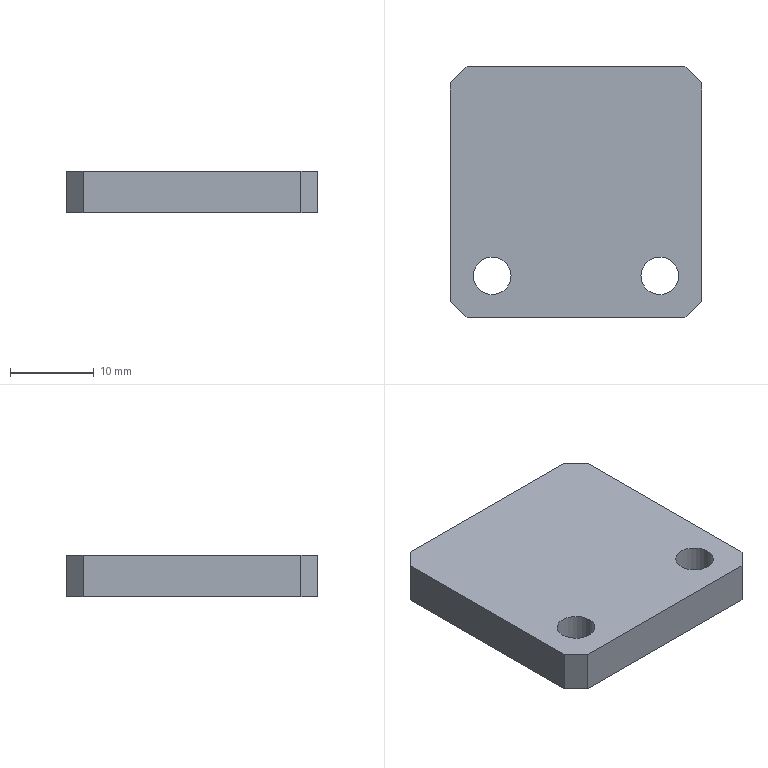Part | STEP file | 01-12 front baffle | 1 solid | 14 faces | box 30 x 30 x 5 mm | volume 4301 mm3 | plane 10 | cylinder 4 | commonest cylinder face diameters 4.5 x4
STEP:
#1=CARTESIAN_POINT('',(7.75,-10.,0.));
#2=VERTEX_POINT('',#1);
#3=CARTESIAN_POINT('',(12.25,-10.,0.));
#4=VERTEX_POINT('',#3);
#5=CARTESIAN_POINT('',(10.,-10.,0.));
#6=DIRECTION('',(0.,0.,1.));
#7=DIRECTION('',(1.,0.,0.));
#8=AXIS2_PLACEMENT_3D('',#5,#6,#7);
#9=CIRCLE('',#8,2.25);
#10=EDGE_CURVE('',#2,#4,#9,.T.);
#11=ORIENTED_EDGE('',*,*,#10,.F.);
#12=CARTESIAN_POINT('',(7.75,-10.,5.));
#13=VERTEX_POINT('',#12);
#14=CARTESIAN_POINT('',(7.75,-10.,0.));
#15=DIRECTION('',(0.,0.,1.));
#16=VECTOR('',#15,1000.);
#17=LINE('',#14,#16);
#18=EDGE_CURVE('',#2,#13,#17,.T.);
#19=ORIENTED_EDGE('',*,*,#18,.T.);
#20=CARTESIAN_POINT('',(12.25,-10.,5.));
#21=VERTEX_POINT('',#20);
#22=CARTESIAN_POINT('',(10.,-10.,5.));
#23=DIRECTION('',(0.,0.,1.));
#24=DIRECTION('',(1.,0.,0.));
#25=AXIS2_PLACEMENT_3D('',#22,#23,#24);
#26=CIRCLE('',#25,2.25);
#27=EDGE_CURVE('',#13,#21,#26,.T.);
#28=ORIENTED_EDGE('',*,*,#27,.T.);
#29=CARTESIAN_POINT('',(12.25,-10.,0.));
#30=DIRECTION('',(0.,0.,1.));
#31=VECTOR('',#30,1000.);
#32=LINE('',#29,#31);
#33=EDGE_CURVE('',#4,#21,#32,.T.);
#34=ORIENTED_EDGE('',*,*,#33,.F.);
#35=EDGE_LOOP('',(#11,#19,#28,#34));
#36=FACE_OUTER_BOUND('',#35,.T.);
#37=CARTESIAN_POINT('',(10.,-10.,0.));
#38=DIRECTION('',(0.,0.,1.));
#39=DIRECTION('',(1.,0.,0.));
#40=AXIS2_PLACEMENT_3D('',#37,#38,#39);
#41=CYLINDRICAL_SURFACE('',#40,2.25);
#42=ADVANCED_FACE('',(#36),#41,.F.);
#43=CARTESIAN_POINT('',(-12.25,-10.,0.));
#44=VERTEX_POINT('',#43);
#45=CARTESIAN_POINT('',(-7.75,-10.,0.));
#46=VERTEX_POINT('',#45);
#47=CARTESIAN_POINT('',(-10.,-10.,0.));
#48=DIRECTION('',(0.,0.,1.));
#49=DIRECTION('',(1.,0.,0.));
#50=AXIS2_PLACEMENT_3D('',#47,#48,#49);
#51=CIRCLE('',#50,2.25);
#52=EDGE_CURVE('',#44,#46,#51,.T.);
#53=ORIENTED_EDGE('',*,*,#52,.F.);
#54=CARTESIAN_POINT('',(-12.25,-10.,5.));
#55=VERTEX_POINT('',#54);
#56=CARTESIAN_POINT('',(-12.25,-10.,0.));
#57=DIRECTION('',(0.,0.,1.));
#58=VECTOR('',#57,1000.);
#59=LINE('',#56,#58);
#60=EDGE_CURVE('',#44,#55,#59,.T.);
#61=ORIENTED_EDGE('',*,*,#60,.T.);
#62=CARTESIAN_POINT('',(-7.75,-10.,5.));
#63=VERTEX_POINT('',#62);
#64=CARTESIAN_POINT('',(-10.,-10.,5.));
#65=DIRECTION('',(0.,0.,1.));
#66=DIRECTION('',(1.,0.,0.));
#67=AXIS2_PLACEMENT_3D('',#64,#65,#66);
#68=CIRCLE('',#67,2.25);
#69=EDGE_CURVE('',#55,#63,#68,.T.);
#70=ORIENTED_EDGE('',*,*,#69,.T.);
#71=CARTESIAN_POINT('',(-7.75,-10.,0.));
#72=DIRECTION('',(0.,0.,1.));
#73=VECTOR('',#72,1000.);
#74=LINE('',#71,#73);
#75=EDGE_CURVE('',#46,#63,#74,.T.);
#76=ORIENTED_EDGE('',*,*,#75,.F.);
#77=EDGE_LOOP('',(#53,#61,#70,#76));
#78=FACE_OUTER_BOUND('',#77,.T.);
#79=CARTESIAN_POINT('',(-10.,-10.,0.));
#80=DIRECTION('',(0.,0.,1.));
#81=DIRECTION('',(1.,0.,0.));
#82=AXIS2_PLACEMENT_3D('',#79,#80,#81);
#83=CYLINDRICAL_SURFACE('',#82,2.25);
#84=ADVANCED_FACE('',(#78),#83,.F.);
#85=CARTESIAN_POINT('',(15.,-13.,5.));
#86=VERTEX_POINT('',#85);
#87=CARTESIAN_POINT('',(15.,13.,5.));
#88=VERTEX_POINT('',#87);
#89=CARTESIAN_POINT('',(15.,15.,5.));
#90=DIRECTION('',(0.,1.,0.));
#91=VECTOR('',#90,1000.);
#92=LINE('',#89,#91);
#93=EDGE_CURVE('',#86,#88,#92,.T.);
#94=ORIENTED_EDGE('',*,*,#93,.F.);
#95=CARTESIAN_POINT('',(15.,-13.,0.));
#96=VERTEX_POINT('',#95);
#97=CARTESIAN_POINT('',(15.,-13.,5.));
#98=DIRECTION('',(0.,0.,-1.));
#99=VECTOR('',#98,1000.);
#100=LINE('',#97,#99);
#101=EDGE_CURVE('',#86,#96,#100,.T.);
#102=ORIENTED_EDGE('',*,*,#101,.T.);
#103=CARTESIAN_POINT('',(15.,13.,0.));
#104=VERTEX_POINT('',#103);
#105=CARTESIAN_POINT('',(15.,15.,0.));
#106=DIRECTION('',(0.,1.,0.));
#107=VECTOR('',#106,1000.);
#108=LINE('',#105,#107);
#109=EDGE_CURVE('',#96,#104,#108,.T.);
#110=ORIENTED_EDGE('',*,*,#109,.T.);
#111=CARTESIAN_POINT('',(15.,13.,5.));
#112=DIRECTION('',(0.,0.,1.));
#113=VECTOR('',#112,1000.);
#114=LINE('',#111,#113);
#115=EDGE_CURVE('',#104,#88,#114,.T.);
#116=ORIENTED_EDGE('',*,*,#115,.T.);
#117=EDGE_LOOP('',(#94,#102,#110,#116));
#118=FACE_OUTER_BOUND('',#117,.T.);
#119=CARTESIAN_POINT('',(15.,15.,5.));
#120=DIRECTION('',(-1.,0.,0.));
#121=DIRECTION('',(0.,-1.,0.));
#122=AXIS2_PLACEMENT_3D('',#119,#120,#121);
#123=PLANE('',#122);
#124=ADVANCED_FACE('',(#118),#123,.F.);
#125=CARTESIAN_POINT('',(13.,15.,5.));
#126=VERTEX_POINT('',#125);
#127=CARTESIAN_POINT('',(-13.,15.,5.));
#128=VERTEX_POINT('',#127);
#129=CARTESIAN_POINT('',(-15.,15.,5.));
#130=DIRECTION('',(-1.,0.,0.));
#131=VECTOR('',#130,1000.);
#132=LINE('',#129,#131);
#133=EDGE_CURVE('',#126,#128,#132,.T.);
#134=ORIENTED_EDGE('',*,*,#133,.F.);
#135=CARTESIAN_POINT('',(13.,15.,0.));
#136=VERTEX_POINT('',#135);
#137=CARTESIAN_POINT('',(13.,15.,5.));
#138=DIRECTION('',(0.,0.,-1.));
#139=VECTOR('',#138,1000.);
#140=LINE('',#137,#139);
#141=EDGE_CURVE('',#126,#136,#140,.T.);
#142=ORIENTED_EDGE('',*,*,#141,.T.);
#143=CARTESIAN_POINT('',(-13.,15.,0.));
#144=VERTEX_POINT('',#143);
#145=CARTESIAN_POINT('',(-15.,15.,0.));
#146=DIRECTION('',(-1.,0.,0.));
#147=VECTOR('',#146,1000.);
#148=LINE('',#145,#147);
#149=EDGE_CURVE('',#136,#144,#148,.T.);
#150=ORIENTED_EDGE('',*,*,#149,.T.);
#151=CARTESIAN_POINT('',(-13.,15.,5.));
#152=DIRECTION('',(0.,0.,1.));
#153=VECTOR('',#152,1000.);
#154=LINE('',#151,#153);
#155=EDGE_CURVE('',#144,#128,#154,.T.);
#156=ORIENTED_EDGE('',*,*,#155,.T.);
#157=EDGE_LOOP('',(#134,#142,#150,#156));
#158=FACE_OUTER_BOUND('',#157,.T.);
#159=CARTESIAN_POINT('',(-15.,15.,5.));
#160=DIRECTION('',(0.,-1.,0.));
#161=DIRECTION('',(0.,0.,-1.));
#162=AXIS2_PLACEMENT_3D('',#159,#160,#161);
#163=PLANE('',#162);
#164=ADVANCED_FACE('',(#158),#163,.F.);
#165=CARTESIAN_POINT('',(-15.,13.,0.));
#166=VERTEX_POINT('',#165);
#167=CARTESIAN_POINT('',(-15.,-13.,0.));
#168=VERTEX_POINT('',#167);
#169=CARTESIAN_POINT('',(-15.,15.,0.));
#170=DIRECTION('',(0.,-1.,0.));
#171=VECTOR('',#170,1000.);
#172=LINE('',#169,#171);
#173=EDGE_CURVE('',#166,#168,#172,.T.);
#174=ORIENTED_EDGE('',*,*,#173,.T.);
#175=CARTESIAN_POINT('',(-15.,-13.,5.));
#176=VERTEX_POINT('',#175);
#177=CARTESIAN_POINT('',(-15.,-13.,5.));
#178=DIRECTION('',(0.,0.,1.));
#179=VECTOR('',#178,1000.);
#180=LINE('',#177,#179);
#181=EDGE_CURVE('',#168,#176,#180,.T.);
#182=ORIENTED_EDGE('',*,*,#181,.T.);
#183=CARTESIAN_POINT('',(-15.,13.,5.));
#184=VERTEX_POINT('',#183);
#185=CARTESIAN_POINT('',(-15.,15.,5.));
#186=DIRECTION('',(0.,-1.,0.));
#187=VECTOR('',#186,1000.);
#188=LINE('',#185,#187);
#189=EDGE_CURVE('',#184,#176,#188,.T.);
#190=ORIENTED_EDGE('',*,*,#189,.F.);
#191=CARTESIAN_POINT('',(-15.,13.,5.));
#192=DIRECTION('',(0.,0.,-1.));
#193=VECTOR('',#192,1000.);
#194=LINE('',#191,#193);
#195=EDGE_CURVE('',#184,#166,#194,.T.);
#196=ORIENTED_EDGE('',*,*,#195,.T.);
#197=EDGE_LOOP('',(#174,#182,#190,#196));
#198=FACE_OUTER_BOUND('',#197,.T.);
#199=CARTESIAN_POINT('',(-15.,15.,5.));
#200=DIRECTION('',(1.,0.,0.));
#201=DIRECTION('',(0.,1.,0.));
#202=AXIS2_PLACEMENT_3D('',#199,#200,#201);
#203=PLANE('',#202);
#204=ADVANCED_FACE('',(#198),#203,.F.);
#205=CARTESIAN_POINT('',(-13.,-15.,0.));
#206=VERTEX_POINT('',#205);
#207=CARTESIAN_POINT('',(13.,-15.,0.));
#208=VERTEX_POINT('',#207);
#209=CARTESIAN_POINT('',(-15.,-15.,0.));
#210=DIRECTION('',(1.,0.,0.));
#211=VECTOR('',#210,1000.);
#212=LINE('',#209,#211);
#213=EDGE_CURVE('',#206,#208,#212,.T.);
#214=ORIENTED_EDGE('',*,*,#213,.T.);
#215=CARTESIAN_POINT('',(13.,-15.,5.));
#216=VERTEX_POINT('',#215);
#217=CARTESIAN_POINT('',(13.,-15.,5.));
#218=DIRECTION('',(0.,0.,1.));
#219=VECTOR('',#218,1000.);
#220=LINE('',#217,#219);
#221=EDGE_CURVE('',#208,#216,#220,.T.);
#222=ORIENTED_EDGE('',*,*,#221,.T.);
#223=CARTESIAN_POINT('',(-13.,-15.,5.));
#224=VERTEX_POINT('',#223);
#225=CARTESIAN_POINT('',(-15.,-15.,5.));
#226=DIRECTION('',(1.,0.,0.));
#227=VECTOR('',#226,1000.);
#228=LINE('',#225,#227);
#229=EDGE_CURVE('',#224,#216,#228,.T.);
#230=ORIENTED_EDGE('',*,*,#229,.F.);
#231=CARTESIAN_POINT('',(-13.,-15.,5.));
#232=DIRECTION('',(0.,0.,-1.));
#233=VECTOR('',#232,1000.);
#234=LINE('',#231,#233);
#235=EDGE_CURVE('',#224,#206,#234,.T.);
#236=ORIENTED_EDGE('',*,*,#235,.T.);
#237=EDGE_LOOP('',(#214,#222,#230,#236));
#238=FACE_OUTER_BOUND('',#237,.T.);
#239=CARTESIAN_POINT('',(-15.,-15.,5.));
#240=DIRECTION('',(0.,1.,0.));
#241=DIRECTION('',(0.,0.,1.));
#242=AXIS2_PLACEMENT_3D('',#239,#240,#241);
#243=PLANE('',#242);
#244=ADVANCED_FACE('',(#238),#243,.F.);
#245=CARTESIAN_POINT('',(10.,-10.,5.));
#246=DIRECTION('',(0.,0.,1.));
#247=DIRECTION('',(1.,0.,0.));
#248=AXIS2_PLACEMENT_3D('',#245,#246,#247);
#249=CIRCLE('',#248,2.25);
#250=EDGE_CURVE('',#21,#13,#249,.T.);
#251=ORIENTED_EDGE('',*,*,#250,.F.);
#252=ORIENTED_EDGE('',*,*,#27,.F.);
#253=EDGE_LOOP('',(#251,#252));
#254=FACE_BOUND('',#253,.T.);
#255=CARTESIAN_POINT('',(-10.,-10.,5.));
#256=DIRECTION('',(0.,0.,1.));
#257=DIRECTION('',(1.,0.,0.));
#258=AXIS2_PLACEMENT_3D('',#255,#256,#257);
#259=CIRCLE('',#258,2.25);
#260=EDGE_CURVE('',#63,#55,#259,.T.);
#261=ORIENTED_EDGE('',*,*,#260,.F.);
#262=ORIENTED_EDGE('',*,*,#69,.F.);
#263=EDGE_LOOP('',(#261,#262));
#264=FACE_BOUND('',#263,.T.);
#265=ORIENTED_EDGE('',*,*,#229,.T.);
#266=CARTESIAN_POINT('',(14.,-14.,5.));
#267=DIRECTION('',(0.7071,0.7071,0.));
#268=VECTOR('',#267,1000.);
#269=LINE('',#266,#268);
#270=EDGE_CURVE('',#216,#86,#269,.T.);
#271=ORIENTED_EDGE('',*,*,#270,.T.);
#272=ORIENTED_EDGE('',*,*,#93,.T.);
#273=CARTESIAN_POINT('',(29.,-1.,5.));
#274=DIRECTION('',(-0.7071,0.7071,0.));
#275=VECTOR('',#274,1000.);
#276=LINE('',#273,#275);
#277=EDGE_CURVE('',#88,#126,#276,.T.);
#278=ORIENTED_EDGE('',*,*,#277,.T.);
#279=ORIENTED_EDGE('',*,*,#133,.T.);
#280=CARTESIAN_POINT('',(-14.,14.,5.));
#281=DIRECTION('',(-0.7071,-0.7071,0.));
#282=VECTOR('',#281,1000.);
#283=LINE('',#280,#282);
#284=EDGE_CURVE('',#128,#184,#283,.T.);
#285=ORIENTED_EDGE('',*,*,#284,.T.);
#286=ORIENTED_EDGE('',*,*,#189,.T.);
#287=CARTESIAN_POINT('',(1.,-29.,5.));
#288=DIRECTION('',(0.7071,-0.7071,0.));
#289=VECTOR('',#288,1000.);
#290=LINE('',#287,#289);
#291=EDGE_CURVE('',#176,#224,#290,.T.);
#292=ORIENTED_EDGE('',*,*,#291,.T.);
#293=EDGE_LOOP('',(#265,#271,#272,#278,#279,#285,#286,#292));
#294=FACE_OUTER_BOUND('',#293,.T.);
#295=CARTESIAN_POINT('',(15.,-15.,5.));
#296=DIRECTION('',(0.,0.,1.));
#297=DIRECTION('',(1.,0.,0.));
#298=AXIS2_PLACEMENT_3D('',#295,#296,#297);
#299=PLANE('',#298);
#300=ADVANCED_FACE('',(#254,#264,#294),#299,.T.);
#301=CARTESIAN_POINT('',(10.,-10.,0.));
#302=DIRECTION('',(0.,0.,1.));
#303=DIRECTION('',(1.,0.,0.));
#304=AXIS2_PLACEMENT_3D('',#301,#302,#303);
#305=CIRCLE('',#304,2.25);
#306=EDGE_CURVE('',#4,#2,#305,.T.);
#307=ORIENTED_EDGE('',*,*,#306,.T.);
#308=ORIENTED_EDGE('',*,*,#10,.T.);
#309=EDGE_LOOP('',(#307,#308));
#310=FACE_BOUND('',#309,.T.);
#311=CARTESIAN_POINT('',(-10.,-10.,0.));
#312=DIRECTION('',(0.,0.,1.));
#313=DIRECTION('',(1.,0.,0.));
#314=AXIS2_PLACEMENT_3D('',#311,#312,#313);
#315=CIRCLE('',#314,2.25);
#316=EDGE_CURVE('',#46,#44,#315,.T.);
#317=ORIENTED_EDGE('',*,*,#316,.T.);
#318=ORIENTED_EDGE('',*,*,#52,.T.);
#319=EDGE_LOOP('',(#317,#318));
#320=FACE_BOUND('',#319,.T.);
#321=ORIENTED_EDGE('',*,*,#109,.F.);
#322=CARTESIAN_POINT('',(15.,-13.,0.));
#323=DIRECTION('',(-0.7071,-0.7071,0.));
#324=VECTOR('',#323,1000.);
#325=LINE('',#322,#324);
#326=EDGE_CURVE('',#96,#208,#325,.T.);
#327=ORIENTED_EDGE('',*,*,#326,.T.);
#328=ORIENTED_EDGE('',*,*,#213,.F.);
#329=CARTESIAN_POINT('',(-13.,-15.,0.));
#330=DIRECTION('',(-0.7071,0.7071,0.));
#331=VECTOR('',#330,1000.);
#332=LINE('',#329,#331);
#333=EDGE_CURVE('',#206,#168,#332,.T.);
#334=ORIENTED_EDGE('',*,*,#333,.T.);
#335=ORIENTED_EDGE('',*,*,#173,.F.);
#336=CARTESIAN_POINT('',(-15.,13.,0.));
#337=DIRECTION('',(0.7071,0.7071,0.));
#338=VECTOR('',#337,1000.);
#339=LINE('',#336,#338);
#340=EDGE_CURVE('',#166,#144,#339,.T.);
#341=ORIENTED_EDGE('',*,*,#340,.T.);
#342=ORIENTED_EDGE('',*,*,#149,.F.);
#343=CARTESIAN_POINT('',(13.,15.,0.));
#344=DIRECTION('',(0.7071,-0.7071,0.));
#345=VECTOR('',#344,1000.);
#346=LINE('',#343,#345);
#347=EDGE_CURVE('',#136,#104,#346,.T.);
#348=ORIENTED_EDGE('',*,*,#347,.T.);
#349=EDGE_LOOP('',(#321,#327,#328,#334,#335,#341,#342,#348));
#350=FACE_OUTER_BOUND('',#349,.T.);
#351=CARTESIAN_POINT('',(15.,-15.,0.));
#352=DIRECTION('',(0.,0.,1.));
#353=DIRECTION('',(1.,0.,0.));
#354=AXIS2_PLACEMENT_3D('',#351,#352,#353);
#355=PLANE('',#354);
#356=ADVANCED_FACE('',(#310,#320,#350),#355,.F.);
#357=ORIENTED_EDGE('',*,*,#270,.F.);
#358=ORIENTED_EDGE('',*,*,#221,.F.);
#359=ORIENTED_EDGE('',*,*,#326,.F.);
#360=ORIENTED_EDGE('',*,*,#101,.F.);
#361=EDGE_LOOP('',(#357,#358,#359,#360));
#362=FACE_OUTER_BOUND('',#361,.T.);
#363=CARTESIAN_POINT('',(15.,-13.,5.));
#364=DIRECTION('',(-0.7071,0.7071,0.));
#365=DIRECTION('',(-0.7071,-0.7071,0.));
#366=AXIS2_PLACEMENT_3D('',#363,#364,#365);
#367=PLANE('',#366);
#368=ADVANCED_FACE('',(#362),#367,.F.);
#369=ORIENTED_EDGE('',*,*,#291,.F.);
#370=ORIENTED_EDGE('',*,*,#181,.F.);
#371=ORIENTED_EDGE('',*,*,#333,.F.);
#372=ORIENTED_EDGE('',*,*,#235,.F.);
#373=EDGE_LOOP('',(#369,#370,#371,#372));
#374=FACE_OUTER_BOUND('',#373,.T.);
#375=CARTESIAN_POINT('',(-13.,-15.,5.));
#376=DIRECTION('',(0.7071,0.7071,0.));
#377=DIRECTION('',(-0.7071,0.7071,0.));
#378=AXIS2_PLACEMENT_3D('',#375,#376,#377);
#379=PLANE('',#378);
#380=ADVANCED_FACE('',(#374),#379,.F.);
#381=ORIENTED_EDGE('',*,*,#277,.F.);
#382=ORIENTED_EDGE('',*,*,#115,.F.);
#383=ORIENTED_EDGE('',*,*,#347,.F.);
#384=ORIENTED_EDGE('',*,*,#141,.F.);
#385=EDGE_LOOP('',(#381,#382,#383,#384));
#386=FACE_OUTER_BOUND('',#385,.T.);
#387=CARTESIAN_POINT('',(13.,15.,5.));
#388=DIRECTION('',(-0.7071,-0.7071,0.));
#389=DIRECTION('',(0.7071,-0.7071,0.));
#390=AXIS2_PLACEMENT_3D('',#387,#388,#389);
#391=PLANE('',#390);
#392=ADVANCED_FACE('',(#386),#391,.F.);
#393=ORIENTED_EDGE('',*,*,#284,.F.);
#394=ORIENTED_EDGE('',*,*,#155,.F.);
#395=ORIENTED_EDGE('',*,*,#340,.F.);
#396=ORIENTED_EDGE('',*,*,#195,.F.);
#397=EDGE_LOOP('',(#393,#394,#395,#396));
#398=FACE_OUTER_BOUND('',#397,.T.);
#399=CARTESIAN_POINT('',(-15.,13.,5.));
#400=DIRECTION('',(0.7071,-0.7071,0.));
#401=DIRECTION('',(0.7071,0.7071,0.));
#402=AXIS2_PLACEMENT_3D('',#399,#400,#401);
#403=PLANE('',#402);
#404=ADVANCED_FACE('',(#398),#403,.F.);
#405=ORIENTED_EDGE('',*,*,#60,.F.);
#406=ORIENTED_EDGE('',*,*,#316,.F.);
#407=ORIENTED_EDGE('',*,*,#75,.T.);
#408=ORIENTED_EDGE('',*,*,#260,.T.);
#409=EDGE_LOOP('',(#405,#406,#407,#408));
#410=FACE_OUTER_BOUND('',#409,.T.);
#411=CARTESIAN_POINT('',(-10.,-10.,0.));
#412=DIRECTION('',(0.,0.,1.));
#413=DIRECTION('',(1.,0.,0.));
#414=AXIS2_PLACEMENT_3D('',#411,#412,#413);
#415=CYLINDRICAL_SURFACE('',#414,2.25);
#416=ADVANCED_FACE('',(#410),#415,.F.);
#417=ORIENTED_EDGE('',*,*,#18,.F.);
#418=ORIENTED_EDGE('',*,*,#306,.F.);
#419=ORIENTED_EDGE('',*,*,#33,.T.);
#420=ORIENTED_EDGE('',*,*,#250,.T.);
#421=EDGE_LOOP('',(#417,#418,#419,#420));
#422=FACE_OUTER_BOUND('',#421,.T.);
#423=CARTESIAN_POINT('',(10.,-10.,0.));
#424=DIRECTION('',(0.,0.,1.));
#425=DIRECTION('',(1.,0.,0.));
#426=AXIS2_PLACEMENT_3D('',#423,#424,#425);
#427=CYLINDRICAL_SURFACE('',#426,2.25);
#428=ADVANCED_FACE('',(#422),#427,.F.);
#429=CLOSED_SHELL('',(#42,#84,#124,#164,#204,#244,#300,#356,#368,#380,#392,#404,#416,#428));
#430=MANIFOLD_SOLID_BREP('',#429);
#431=CARTESIAN_POINT('',(0.,0.,0.));
#432=DIRECTION('',(0.,0.,1.));
#433=DIRECTION('',(1.,0.,0.));
#434=AXIS2_PLACEMENT_3D('',#431,#432,#433);
#435=(LENGTH_UNIT()NAMED_UNIT(*)SI_UNIT(.MILLI.,.METRE.));
#436=UNCERTAINTY_MEASURE_WITH_UNIT(LENGTH_MEASURE(0.00001),#435,'','');
#437=(NAMED_UNIT(*)PLANE_ANGLE_UNIT()SI_UNIT($,.RADIAN.));
#438=(NAMED_UNIT(*)SI_UNIT($,.STERADIAN.)SOLID_ANGLE_UNIT());
#439=(GEOMETRIC_REPRESENTATION_CONTEXT(3)GLOBAL_UNCERTAINTY_ASSIGNED_CONTEXT((#436))GLOBAL_UNIT_ASSIGNED_CONTEXT((#435,#437,#438))REPRESENTATION_CONTEXT('',''));
#440=ADVANCED_BREP_SHAPE_REPRESENTATION('',(#430,#434),#439);